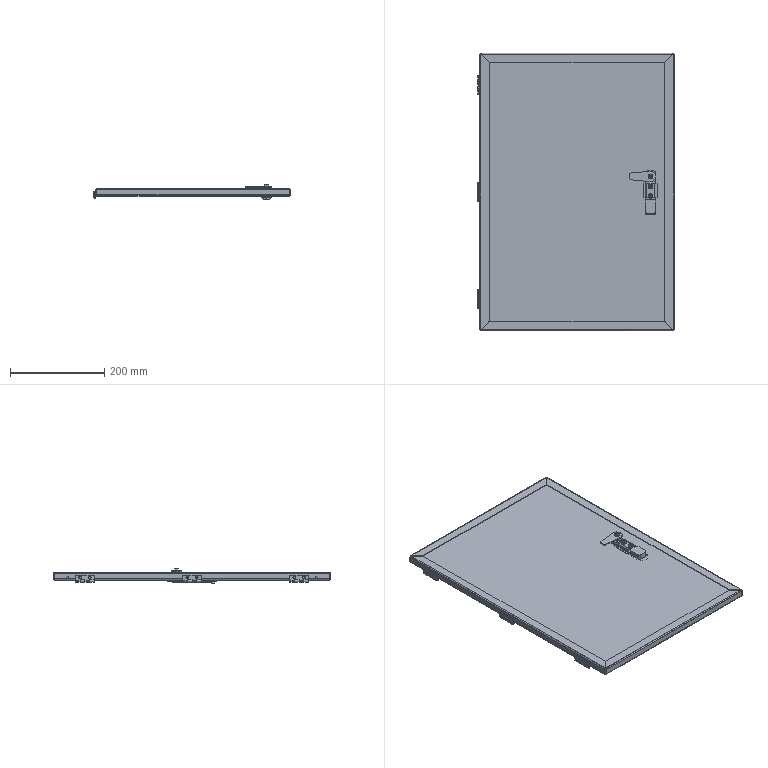Part | SolidWorks | 8 solids | 434 faces | box 415.8 x 588 x 32.227 mm | volume 489087 mm3 | plane 230 | cylinder 141 | cone 45 | spline 18 | commonest cylinder face diameters 4.3 x36 2 x32 3.3 x12 10 x10 1.473 x8 4.473 x8